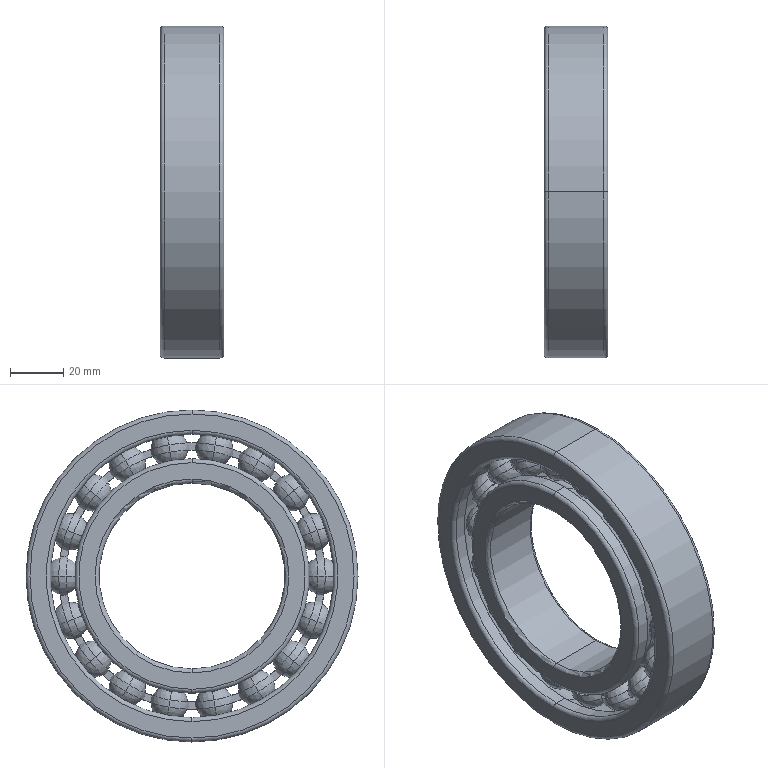Part | SolidWorks | features Revolution 4, CirPattern 2, RefAxis 1, RevCut 1 | 20 solids | 220 faces | box 24 x 125 x 125 mm | volume 151869 mm3 | cylinder 82 | sphere 76 | plane 40 | torus 22 | commonest cylinder face diameters 94.75 x35 100.25 x35 88.333 x4 106.667 x4 70 x2 125 x2